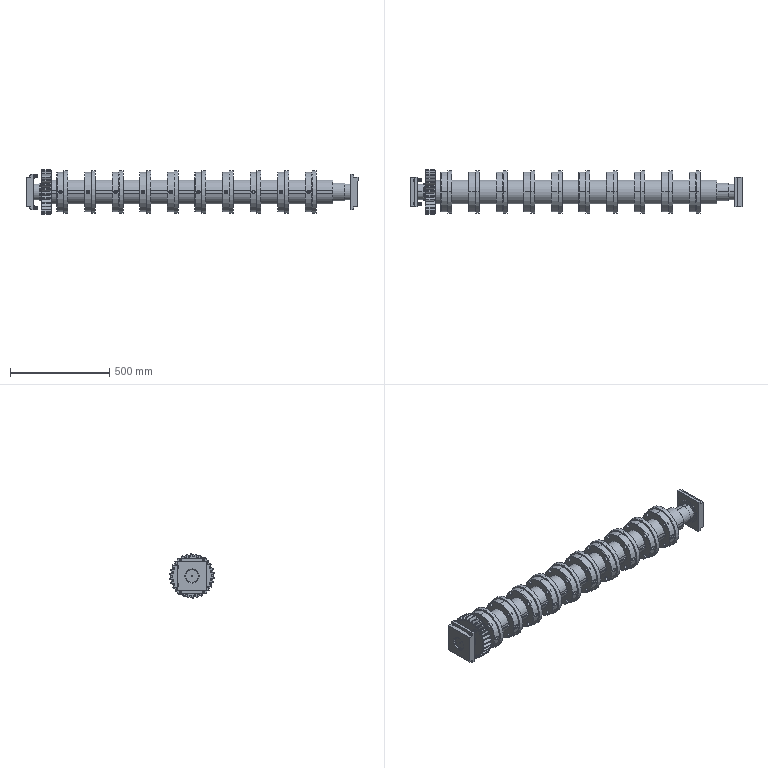Part | SolidWorks | 70 solids | 1743 faces | box 1672 x 223.661 x 223.999 mm | volume 30966531 mm3 | cylinder 719 | plane 414 | cone 346 | sphere 144 | torus 60 | spline 60 | commonest cylinder face diameters 20 x82 10.2 x80 13 x80 89.75 x66 95.25 x66 120 x41